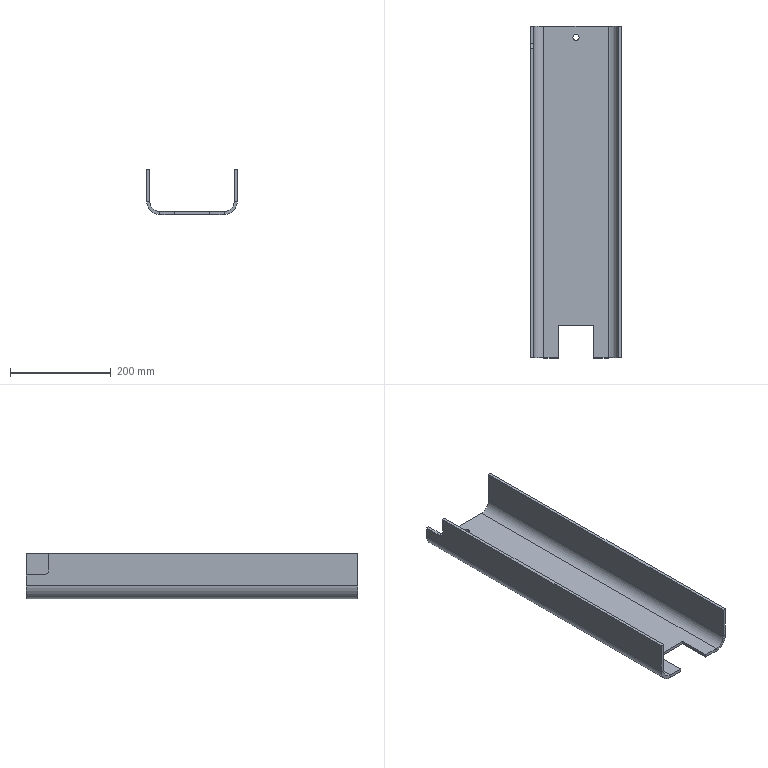Part | SolidWorks | features Cut 1, FlatPattern 1, SM3dBend 1, SMBaseFlange 1, SheetMetal 1 | 1 solid | 31 faces | box 180.012 x 660 x 89.996 mm | volume 1260450 mm3 | plane 24 | cylinder 7 | commonest cylinder face diameters 12 x2 40 x2 52 x2 20 x1
STEP:
#1=CARTESIAN_POINT('',(158.126,637.5,-6.));
#2=VERTEX_POINT('',#1);
#3=CARTESIAN_POINT('',(170.126,637.5,-6.));
#4=VERTEX_POINT('',#3);
#5=CARTESIAN_POINT('',(164.126,637.5,-6.));
#6=DIRECTION('',(0.,0.,1.));
#7=DIRECTION('',(1.,0.,0.));
#8=AXIS2_PLACEMENT_3D('',#5,#6,#7);
#9=CIRCLE('',#8,6.);
#10=EDGE_CURVE('',#2,#4,#9,.T.);
#11=ORIENTED_EDGE('',*,*,#10,.F.);
#12=CARTESIAN_POINT('',(158.126,637.5,0.));
#13=VERTEX_POINT('',#12);
#14=CARTESIAN_POINT('',(158.126,637.5,-6.));
#15=DIRECTION('',(0.,0.,1.));
#16=VECTOR('',#15,1000.);
#17=LINE('',#14,#16);
#18=EDGE_CURVE('',#2,#13,#17,.T.);
#19=ORIENTED_EDGE('',*,*,#18,.T.);
#20=CARTESIAN_POINT('',(170.126,637.5,0.));
#21=VERTEX_POINT('',#20);
#22=CARTESIAN_POINT('',(164.126,637.5,0.));
#23=DIRECTION('',(0.,0.,1.));
#24=DIRECTION('',(1.,0.,0.));
#25=AXIS2_PLACEMENT_3D('',#22,#23,#24);
#26=CIRCLE('',#25,6.);
#27=EDGE_CURVE('',#13,#21,#26,.T.);
#28=ORIENTED_EDGE('',*,*,#27,.T.);
#29=CARTESIAN_POINT('',(170.126,637.5,-6.));
#30=DIRECTION('',(0.,0.,1.));
#31=VECTOR('',#30,1000.);
#32=LINE('',#29,#31);
#33=EDGE_CURVE('',#4,#21,#32,.T.);
#34=ORIENTED_EDGE('',*,*,#33,.F.);
#35=EDGE_LOOP('',(#11,#19,#28,#34));
#36=FACE_OUTER_BOUND('',#35,.T.);
#37=CARTESIAN_POINT('',(164.126,637.5,-6.));
#38=DIRECTION('',(0.,0.,1.));
#39=DIRECTION('',(1.,0.,0.));
#40=AXIS2_PLACEMENT_3D('',#37,#38,#39);
#41=CYLINDRICAL_SURFACE('',#40,6.);
#42=ADVANCED_FACE('',(#36),#41,.F.);
#43=CARTESIAN_POINT('',(164.126,637.5,-6.));
#44=DIRECTION('',(0.,0.,1.));
#45=DIRECTION('',(1.,0.,0.));
#46=AXIS2_PLACEMENT_3D('',#43,#44,#45);
#47=CIRCLE('',#46,6.);
#48=EDGE_CURVE('',#4,#2,#47,.T.);
#49=ORIENTED_EDGE('',*,*,#48,.T.);
#50=ORIENTED_EDGE('',*,*,#10,.T.);
#51=EDGE_LOOP('',(#49,#50));
#52=FACE_BOUND('',#51,.T.);
#53=CARTESIAN_POINT('',(228.136,660.,-6.));
#54=VERTEX_POINT('',#53);
#55=CARTESIAN_POINT('',(100.124,660.,-6.));
#56=VERTEX_POINT('',#55);
#57=CARTESIAN_POINT('',(328.26,660.,-6.));
#58=DIRECTION('',(-1.,0.,0.));
#59=VECTOR('',#58,1000.);
#60=LINE('',#57,#59);
#61=EDGE_CURVE('',#54,#56,#60,.T.);
#62=ORIENTED_EDGE('',*,*,#61,.F.);
#63=CARTESIAN_POINT('',(228.136,0.,-6.));
#64=VERTEX_POINT('',#63);
#65=CARTESIAN_POINT('',(228.136,625.,-6.));
#66=DIRECTION('',(0.,-1.,0.));
#67=VECTOR('',#66,1000.);
#68=LINE('',#65,#67);
#69=EDGE_CURVE('',#54,#64,#68,.T.);
#70=ORIENTED_EDGE('',*,*,#69,.T.);
#71=CARTESIAN_POINT('',(199.13,0.,-6.));
#72=VERTEX_POINT('',#71);
#73=CARTESIAN_POINT('',(199.13,0.,-6.));
#74=DIRECTION('',(1.,0.,0.));
#75=VECTOR('',#74,1000.);
#76=LINE('',#73,#75);
#77=EDGE_CURVE('',#72,#64,#76,.T.);
#78=ORIENTED_EDGE('',*,*,#77,.F.);
#79=CARTESIAN_POINT('',(199.13,65.,-6.));
#80=VERTEX_POINT('',#79);
#81=CARTESIAN_POINT('',(199.13,0.,-6.));
#82=DIRECTION('',(0.,-1.,0.));
#83=VECTOR('',#82,1000.);
#84=LINE('',#81,#83);
#85=EDGE_CURVE('',#80,#72,#84,.T.);
#86=ORIENTED_EDGE('',*,*,#85,.F.);
#87=CARTESIAN_POINT('',(129.13,65.,-6.));
#88=VERTEX_POINT('',#87);
#89=CARTESIAN_POINT('',(199.13,65.,-6.));
#90=DIRECTION('',(1.,0.,0.));
#91=VECTOR('',#90,1000.);
#92=LINE('',#89,#91);
#93=EDGE_CURVE('',#88,#80,#92,.T.);
#94=ORIENTED_EDGE('',*,*,#93,.F.);
#95=CARTESIAN_POINT('',(129.13,0.,-6.));
#96=VERTEX_POINT('',#95);
#97=CARTESIAN_POINT('',(129.13,65.,-6.));
#98=DIRECTION('',(0.,1.,0.));
#99=VECTOR('',#98,1000.);
#100=LINE('',#97,#99);
#101=EDGE_CURVE('',#96,#88,#100,.T.);
#102=ORIENTED_EDGE('',*,*,#101,.F.);
#103=CARTESIAN_POINT('',(100.124,0.,-6.));
#104=VERTEX_POINT('',#103);
#105=CARTESIAN_POINT('',(0.,0.,-6.));
#106=DIRECTION('',(1.,0.,0.));
#107=VECTOR('',#106,1000.);
#108=LINE('',#105,#107);
#109=EDGE_CURVE('',#104,#96,#108,.T.);
#110=ORIENTED_EDGE('',*,*,#109,.F.);
#111=CARTESIAN_POINT('',(100.124,625.,-6.));
#112=DIRECTION('',(0.,-1.,0.));
#113=VECTOR('',#112,1000.);
#114=LINE('',#111,#113);
#115=EDGE_CURVE('',#56,#104,#114,.T.);
#116=ORIENTED_EDGE('',*,*,#115,.F.);
#117=EDGE_LOOP('',(#62,#70,#78,#86,#94,#102,#110,#116));
#118=FACE_OUTER_BOUND('',#117,.T.);
#119=CARTESIAN_POINT('',(33.,625.,-6.));
#120=DIRECTION('',(0.,0.,1.));
#121=DIRECTION('',(1.,0.,0.));
#122=AXIS2_PLACEMENT_3D('',#119,#120,#121);
#123=PLANE('',#122);
#124=ADVANCED_FACE('',(#52,#118),#123,.F.);
#125=CARTESIAN_POINT('',(228.136,660.,0.));
#126=VERTEX_POINT('',#125);
#127=CARTESIAN_POINT('',(228.136,660.,-6.));
#128=DIRECTION('',(0.,0.,1.));
#129=VECTOR('',#128,1000.);
#130=LINE('',#127,#129);
#131=EDGE_CURVE('',#54,#126,#130,.T.);
#132=ORIENTED_EDGE('',*,*,#131,.F.);
#133=ORIENTED_EDGE('',*,*,#61,.T.);
#134=CARTESIAN_POINT('',(100.124,660.,0.));
#135=VERTEX_POINT('',#134);
#136=CARTESIAN_POINT('',(100.124,660.,-6.));
#137=DIRECTION('',(0.,0.,1.));
#138=VECTOR('',#137,1000.);
#139=LINE('',#136,#138);
#140=EDGE_CURVE('',#56,#135,#139,.T.);
#141=ORIENTED_EDGE('',*,*,#140,.T.);
#142=CARTESIAN_POINT('',(328.26,660.,0.));
#143=DIRECTION('',(-1.,0.,0.));
#144=VECTOR('',#143,1000.);
#145=LINE('',#142,#144);
#146=EDGE_CURVE('',#126,#135,#145,.T.);
#147=ORIENTED_EDGE('',*,*,#146,.F.);
#148=EDGE_LOOP('',(#132,#133,#141,#147));
#149=FACE_OUTER_BOUND('',#148,.T.);
#150=CARTESIAN_POINT('',(328.26,660.,-6.));
#151=DIRECTION('',(0.,1.,0.));
#152=DIRECTION('',(0.,0.,1.));
#153=AXIS2_PLACEMENT_3D('',#150,#151,#152);
#154=PLANE('',#153);
#155=ADVANCED_FACE('',(#149),#154,.T.);
#156=CARTESIAN_POINT('',(100.124,0.,0.));
#157=VERTEX_POINT('',#156);
#158=CARTESIAN_POINT('',(129.13,0.,0.));
#159=VERTEX_POINT('',#158);
#160=CARTESIAN_POINT('',(0.,0.,0.));
#161=DIRECTION('',(1.,0.,0.));
#162=VECTOR('',#161,1000.);
#163=LINE('',#160,#162);
#164=EDGE_CURVE('',#157,#159,#163,.T.);
#165=ORIENTED_EDGE('',*,*,#164,.F.);
#166=CARTESIAN_POINT('',(100.124,0.,-6.));
#167=DIRECTION('',(0.,0.,-1.));
#168=VECTOR('',#167,1000.);
#169=LINE('',#166,#168);
#170=EDGE_CURVE('',#157,#104,#169,.T.);
#171=ORIENTED_EDGE('',*,*,#170,.T.);
#172=ORIENTED_EDGE('',*,*,#109,.T.);
#173=CARTESIAN_POINT('',(129.13,0.,-6.));
#174=DIRECTION('',(0.,0.,1.));
#175=VECTOR('',#174,1000.);
#176=LINE('',#173,#175);
#177=EDGE_CURVE('',#96,#159,#176,.T.);
#178=ORIENTED_EDGE('',*,*,#177,.T.);
#179=EDGE_LOOP('',(#165,#171,#172,#178));
#180=FACE_OUTER_BOUND('',#179,.T.);
#181=CARTESIAN_POINT('',(0.,0.,-6.));
#182=DIRECTION('',(0.,-1.,0.));
#183=DIRECTION('',(0.,0.,-1.));
#184=AXIS2_PLACEMENT_3D('',#181,#182,#183);
#185=PLANE('',#184);
#186=ADVANCED_FACE('',(#180),#185,.T.);
#187=CARTESIAN_POINT('',(164.126,637.5,0.));
#188=DIRECTION('',(0.,0.,1.));
#189=DIRECTION('',(1.,0.,0.));
#190=AXIS2_PLACEMENT_3D('',#187,#188,#189);
#191=CIRCLE('',#190,6.);
#192=EDGE_CURVE('',#21,#13,#191,.T.);
#193=ORIENTED_EDGE('',*,*,#192,.F.);
#194=ORIENTED_EDGE('',*,*,#27,.F.);
#195=EDGE_LOOP('',(#193,#194));
#196=FACE_BOUND('',#195,.T.);
#197=CARTESIAN_POINT('',(228.136,0.,0.));
#198=VERTEX_POINT('',#197);
#199=CARTESIAN_POINT('',(228.136,625.,0.));
#200=DIRECTION('',(0.,-1.,0.));
#201=VECTOR('',#200,1000.);
#202=LINE('',#199,#201);
#203=EDGE_CURVE('',#126,#198,#202,.T.);
#204=ORIENTED_EDGE('',*,*,#203,.F.);
#205=ORIENTED_EDGE('',*,*,#146,.T.);
#206=CARTESIAN_POINT('',(100.124,625.,0.));
#207=DIRECTION('',(0.,-1.,0.));
#208=VECTOR('',#207,1000.);
#209=LINE('',#206,#208);
#210=EDGE_CURVE('',#135,#157,#209,.T.);
#211=ORIENTED_EDGE('',*,*,#210,.T.);
#212=ORIENTED_EDGE('',*,*,#164,.T.);
#213=CARTESIAN_POINT('',(129.13,65.,0.));
#214=VERTEX_POINT('',#213);
#215=CARTESIAN_POINT('',(129.13,65.,0.));
#216=DIRECTION('',(0.,1.,0.));
#217=VECTOR('',#216,1000.);
#218=LINE('',#215,#217);
#219=EDGE_CURVE('',#159,#214,#218,.T.);
#220=ORIENTED_EDGE('',*,*,#219,.T.);
#221=CARTESIAN_POINT('',(199.13,65.,0.));
#222=VERTEX_POINT('',#221);
#223=CARTESIAN_POINT('',(199.13,65.,0.));
#224=DIRECTION('',(1.,0.,0.));
#225=VECTOR('',#224,1000.);
#226=LINE('',#223,#225);
#227=EDGE_CURVE('',#214,#222,#226,.T.);
#228=ORIENTED_EDGE('',*,*,#227,.T.);
#229=CARTESIAN_POINT('',(199.13,0.,0.));
#230=VERTEX_POINT('',#229);
#231=CARTESIAN_POINT('',(199.13,0.,0.));
#232=DIRECTION('',(0.,-1.,0.));
#233=VECTOR('',#232,1000.);
#234=LINE('',#231,#233);
#235=EDGE_CURVE('',#222,#230,#234,.T.);
#236=ORIENTED_EDGE('',*,*,#235,.T.);
#237=CARTESIAN_POINT('',(199.13,0.,0.));
#238=DIRECTION('',(1.,0.,0.));
#239=VECTOR('',#238,1000.);
#240=LINE('',#237,#239);
#241=EDGE_CURVE('',#230,#198,#240,.T.);
#242=ORIENTED_EDGE('',*,*,#241,.T.);
#243=EDGE_LOOP('',(#204,#205,#211,#212,#220,#228,#236,#242));
#244=FACE_OUTER_BOUND('',#243,.T.);
#245=CARTESIAN_POINT('',(33.,625.,0.));
#246=DIRECTION('',(0.,0.,1.));
#247=DIRECTION('',(1.,0.,0.));
#248=AXIS2_PLACEMENT_3D('',#245,#246,#247);
#249=PLANE('',#248);
#250=ADVANCED_FACE('',(#196,#244),#249,.T.);
#251=CARTESIAN_POINT('',(228.136,0.,-6.));
#252=DIRECTION('',(0.,0.,-1.));
#253=VECTOR('',#252,1000.);
#254=LINE('',#251,#253);
#255=EDGE_CURVE('',#198,#64,#254,.T.);
#256=ORIENTED_EDGE('',*,*,#255,.F.);
#257=ORIENTED_EDGE('',*,*,#241,.F.);
#258=CARTESIAN_POINT('',(199.13,0.,-6.));
#259=DIRECTION('',(0.,0.,1.));
#260=VECTOR('',#259,1000.);
#261=LINE('',#258,#260);
#262=EDGE_CURVE('',#72,#230,#261,.T.);
#263=ORIENTED_EDGE('',*,*,#262,.F.);
#264=ORIENTED_EDGE('',*,*,#77,.T.);
#265=EDGE_LOOP('',(#256,#257,#263,#264));
#266=FACE_OUTER_BOUND('',#265,.T.);
#267=CARTESIAN_POINT('',(199.13,0.,-6.));
#268=DIRECTION('',(0.,-1.,0.));
#269=DIRECTION('',(0.,0.,-1.));
#270=AXIS2_PLACEMENT_3D('',#267,#268,#269);
#271=PLANE('',#270);
#272=ADVANCED_FACE('',(#266),#271,.T.);
#273=ORIENTED_EDGE('',*,*,#235,.F.);
#274=CARTESIAN_POINT('',(199.13,65.,-6.));
#275=DIRECTION('',(0.,0.,1.));
#276=VECTOR('',#275,1000.);
#277=LINE('',#274,#276);
#278=EDGE_CURVE('',#80,#222,#277,.T.);
#279=ORIENTED_EDGE('',*,*,#278,.F.);
#280=ORIENTED_EDGE('',*,*,#85,.T.);
#281=ORIENTED_EDGE('',*,*,#262,.T.);
#282=EDGE_LOOP('',(#273,#279,#280,#281));
#283=FACE_OUTER_BOUND('',#282,.T.);
#284=CARTESIAN_POINT('',(199.13,0.,-6.));
#285=DIRECTION('',(-1.,0.,0.));
#286=DIRECTION('',(0.,0.,1.));
#287=AXIS2_PLACEMENT_3D('',#284,#285,#286);
#288=PLANE('',#287);
#289=ADVANCED_FACE('',(#283),#288,.T.);
#290=ORIENTED_EDGE('',*,*,#227,.F.);
#291=CARTESIAN_POINT('',(129.13,65.,-6.));
#292=DIRECTION('',(0.,0.,1.));
#293=VECTOR('',#292,1000.);
#294=LINE('',#291,#293);
#295=EDGE_CURVE('',#88,#214,#294,.T.);
#296=ORIENTED_EDGE('',*,*,#295,.F.);
#297=ORIENTED_EDGE('',*,*,#93,.T.);
#298=ORIENTED_EDGE('',*,*,#278,.T.);
#299=EDGE_LOOP('',(#290,#296,#297,#298));
#300=FACE_OUTER_BOUND('',#299,.T.);
#301=CARTESIAN_POINT('',(199.13,65.,-6.));
#302=DIRECTION('',(0.,-1.,0.));
#303=DIRECTION('',(1.,0.,0.));
#304=AXIS2_PLACEMENT_3D('',#301,#302,#303);
#305=PLANE('',#304);
#306=ADVANCED_FACE('',(#300),#305,.T.);
#307=ORIENTED_EDGE('',*,*,#219,.F.);
#308=ORIENTED_EDGE('',*,*,#177,.F.);
#309=ORIENTED_EDGE('',*,*,#101,.T.);
#310=ORIENTED_EDGE('',*,*,#295,.T.);
#311=EDGE_LOOP('',(#307,#308,#309,#310));
#312=FACE_OUTER_BOUND('',#311,.T.);
#313=CARTESIAN_POINT('',(129.13,65.,-6.));
#314=DIRECTION('',(1.,0.,0.));
#315=DIRECTION('',(0.,0.,-1.));
#316=AXIS2_PLACEMENT_3D('',#313,#314,#315);
#317=PLANE('',#316);
#318=ADVANCED_FACE('',(#312),#317,.T.);
#319=CARTESIAN_POINT('',(74.124,660.,20.));
#320=VERTEX_POINT('',#319);
#321=CARTESIAN_POINT('',(80.124,660.,20.));
#322=VERTEX_POINT('',#321);
#323=CARTESIAN_POINT('',(74.124,660.,20.));
#324=DIRECTION('',(1.,0.,0.));
#325=VECTOR('',#324,1000.);
#326=LINE('',#323,#325);
#327=EDGE_CURVE('',#320,#322,#326,.T.);
#328=ORIENTED_EDGE('',*,*,#327,.T.);
#329=CARTESIAN_POINT('',(100.124,660.,20.));
#330=DIRECTION('',(0.,-1.,0.));
#331=DIRECTION('',(0.,0.,1.));
#332=AXIS2_PLACEMENT_3D('',#329,#330,#331);
#333=CIRCLE('',#332,20.);
#334=EDGE_CURVE('',#322,#135,#333,.T.);
#335=ORIENTED_EDGE('',*,*,#334,.T.);
#336=ORIENTED_EDGE('',*,*,#140,.F.);
#337=CARTESIAN_POINT('',(100.124,660.,20.));
#338=DIRECTION('',(0.,-1.,0.));
#339=DIRECTION('',(0.,0.,1.));
#340=AXIS2_PLACEMENT_3D('',#337,#338,#339);
#341=CIRCLE('',#340,26.);
#342=EDGE_CURVE('',#320,#56,#341,.T.);
#343=ORIENTED_EDGE('',*,*,#342,.F.);
#344=EDGE_LOOP('',(#328,#335,#336,#343));
#345=FACE_OUTER_BOUND('',#344,.T.);
#346=CARTESIAN_POINT('',(100.124,660.,20.));
#347=DIRECTION('',(0.,1.,0.));
#348=DIRECTION('',(0.,0.,1.));
#349=AXIS2_PLACEMENT_3D('',#346,#347,#348);
#350=PLANE('',#349);
#351=ADVANCED_FACE('',(#345),#350,.T.);
#352=ORIENTED_EDGE('',*,*,#170,.F.);
#353=CARTESIAN_POINT('',(80.124,0.,20.));
#354=VERTEX_POINT('',#353);
#355=CARTESIAN_POINT('',(100.124,0.,20.));
#356=DIRECTION('',(0.,1.,0.));
#357=DIRECTION('',(0.,0.,1.));
#358=AXIS2_PLACEMENT_3D('',#355,#356,#357);
#359=CIRCLE('',#358,20.);
#360=EDGE_CURVE('',#157,#354,#359,.T.);
#361=ORIENTED_EDGE('',*,*,#360,.T.);
#362=CARTESIAN_POINT('',(74.124,0.,20.));
#363=VERTEX_POINT('',#362);
#364=CARTESIAN_POINT('',(74.124,0.,20.));
#365=DIRECTION('',(-1.,0.,0.));
#366=VECTOR('',#365,1000.);
#367=LINE('',#364,#366);
#368=EDGE_CURVE('',#354,#363,#367,.T.);
#369=ORIENTED_EDGE('',*,*,#368,.T.);
#370=CARTESIAN_POINT('',(100.124,0.,20.));
#371=DIRECTION('',(0.,1.,0.));
#372=DIRECTION('',(0.,0.,-1.));
#373=AXIS2_PLACEMENT_3D('',#370,#371,#372);
#374=CIRCLE('',#373,26.);
#375=EDGE_CURVE('',#104,#363,#374,.T.);
#376=ORIENTED_EDGE('',*,*,#375,.F.);
#377=EDGE_LOOP('',(#352,#361,#369,#376));
#378=FACE_OUTER_BOUND('',#377,.T.);
#379=CARTESIAN_POINT('',(100.124,0.,20.));
#380=DIRECTION('',(0.,-1.,0.));
#381=DIRECTION('',(0.,0.,-1.));
#382=AXIS2_PLACEMENT_3D('',#379,#380,#381);
#383=PLANE('',#382);
#384=ADVANCED_FACE('',(#378),#383,.T.);
#385=ORIENTED_EDGE('',*,*,#375,.T.);
#386=CARTESIAN_POINT('',(74.124,625.,20.));
#387=DIRECTION('',(0.,-1.,0.));
#388=VECTOR('',#387,1000.);
#389=LINE('',#386,#388);
#390=EDGE_CURVE('',#320,#363,#389,.T.);
#391=ORIENTED_EDGE('',*,*,#390,.F.);
#392=ORIENTED_EDGE('',*,*,#342,.T.);
#393=ORIENTED_EDGE('',*,*,#115,.T.);
#394=EDGE_LOOP('',(#385,#391,#392,#393));
#395=FACE_OUTER_BOUND('',#394,.T.);
#396=CARTESIAN_POINT('',(100.124,-331.015,20.));
#397=DIRECTION('',(0.,1.,0.));
#398=DIRECTION('',(0.,0.,1.));
#399=AXIS2_PLACEMENT_3D('',#396,#397,#398);
#400=CYLINDRICAL_SURFACE('',#399,26.);
#401=ADVANCED_FACE('',(#395),#400,.T.);
#402=ORIENTED_EDGE('',*,*,#360,.F.);
#403=ORIENTED_EDGE('',*,*,#210,.F.);
#404=ORIENTED_EDGE('',*,*,#334,.F.);
#405=CARTESIAN_POINT('',(80.124,625.,20.));
#406=DIRECTION('',(0.,-1.,0.));
#407=VECTOR('',#406,1000.);
#408=LINE('',#405,#407);
#409=EDGE_CURVE('',#322,#354,#408,.T.);
#410=ORIENTED_EDGE('',*,*,#409,.T.);
#411=EDGE_LOOP('',(#402,#403,#404,#410));
#412=FACE_OUTER_BOUND('',#411,.T.);
#413=CARTESIAN_POINT('',(100.124,-331.015,20.));
#414=DIRECTION('',(0.,1.,0.));
#415=DIRECTION('',(0.,0.,1.));
#416=AXIS2_PLACEMENT_3D('',#413,#414,#415);
#417=CYLINDRICAL_SURFACE('',#416,20.);
#418=ADVANCED_FACE('',(#412),#417,.F.);
#419=CARTESIAN_POINT('',(80.124,660.,40.996));
#420=VERTEX_POINT('',#419);
#421=CARTESIAN_POINT('',(80.124,625.,40.996));
#422=VERTEX_POINT('',#421);
#423=CARTESIAN_POINT('',(80.124,625.,40.996));
#424=DIRECTION('',(0.,-1.,0.));
#425=VECTOR('',#424,1000.);
#426=LINE('',#423,#425);
#427=EDGE_CURVE('',#420,#422,#426,.T.);
#428=ORIENTED_EDGE('',*,*,#427,.F.);
#429=CARTESIAN_POINT('',(74.124,660.,40.996));
#430=VERTEX_POINT('',#429);
#431=CARTESIAN_POINT('',(74.124,660.,40.996));
#432=DIRECTION('',(1.,0.,0.));
#433=VECTOR('',#432,1000.);
#434=LINE('',#431,#433);
#435=EDGE_CURVE('',#430,#420,#434,.T.);
#436=ORIENTED_EDGE('',*,*,#435,.F.);
#437=CARTESIAN_POINT('',(74.124,625.,40.996));
#438=VERTEX_POINT('',#437);
#439=CARTESIAN_POINT('',(74.124,625.,40.996));
#440=DIRECTION('',(0.,-1.,0.));
#441=VECTOR('',#440,1000.);
#442=LINE('',#439,#441);
#443=EDGE_CURVE('',#430,#438,#442,.T.);
#444=ORIENTED_EDGE('',*,*,#443,.T.);
#445=CARTESIAN_POINT('',(74.124,625.,40.996));
#446=DIRECTION('',(1.,0.,0.));
#447=VECTOR('',#446,1000.);
#448=LINE('',#445,#447);
#449=EDGE_CURVE('',#438,#422,#448,.T.);
#450=ORIENTED_EDGE('',*,*,#449,.T.);
#451=EDGE_LOOP('',(#428,#436,#444,#450));
#452=FACE_OUTER_BOUND('',#451,.T.);
#453=CARTESIAN_POINT('',(74.124,625.,40.996));
#454=DIRECTION('',(0.,0.,1.));
#455=DIRECTION('',(0.,-1.,0.));
#456=AXIS2_PLACEMENT_3D('',#453,#454,#455);
#457=PLANE('',#456);
#458=ADVANCED_FACE('',(#452),#457,.T.);
#459=CARTESIAN_POINT('',(80.124,615.,50.996));
#460=VERTEX_POINT('',#459);
#461=CARTESIAN_POINT('',(80.124,625.,50.996));
#462=DIRECTION('',(-1.,0.,0.));
#463=DIRECTION('',(0.,0.,-1.));
#464=AXIS2_PLACEMENT_3D('',#461,#462,#463);
#465=CIRCLE('',#464,10.);
#466=EDGE_CURVE('',#422,#460,#465,.T.);
#467=ORIENTED_EDGE('',*,*,#466,.F.);
#468=ORIENTED_EDGE('',*,*,#449,.F.);
#469=CARTESIAN_POINT('',(74.124,615.,50.996));
#470=VERTEX_POINT('',#469);
#471=CARTESIAN_POINT('',(74.124,625.,50.996));
#472=DIRECTION('',(-1.,0.,0.));
#473=DIRECTION('',(0.,0.,-1.));
#474=AXIS2_PLACEMENT_3D('',#471,#472,#473);
#475=CIRCLE('',#474,10.);
#476=EDGE_CURVE('',#438,#470,#475,.T.);
#477=ORIENTED_EDGE('',*,*,#476,.T.);
#478=CARTESIAN_POINT('',(74.124,615.,50.996));
#479=DIRECTION('',(1.,0.,0.));
#480=VECTOR('',#479,1000.);
#481=LINE('',#478,#480);
#482=EDGE_CURVE('',#470,#460,#481,.T.);
#483=ORIENTED_EDGE('',*,*,#482,.T.);
#484=EDGE_LOOP('',(#467,#468,#477,#483));
#485=FACE_OUTER_BOUND('',#484,.T.);
#486=CARTESIAN_POINT('',(74.124,625.,50.996));
#487=DIRECTION('',(1.,0.,0.));
#488=DIRECTION('',(0.,0.,-1.));
#489=AXIS2_PLACEMENT_3D('',#486,#487,#488);
#490=CYLINDRICAL_SURFACE('',#489,10.);
#491=ADVANCED_FACE('',(#485),#490,.F.);
#492=CARTESIAN_POINT('',(80.124,615.,83.996));
#493=VERTEX_POINT('',#492);
#494=CARTESIAN_POINT('',(80.124,615.,83.996));
#495=DIRECTION('',(0.,0.,1.));
#496=VECTOR('',#495,1000.);
#497=LINE('',#494,#496);
#498=EDGE_CURVE('',#460,#493,#497,.T.);
#499=ORIENTED_EDGE('',*,*,#498,.F.);
#500=ORIENTED_EDGE('',*,*,#482,.F.);
#501=CARTESIAN_POINT('',(74.124,615.,83.996));
#502=VERTEX_POINT('',#501);
#503=CARTESIAN_POINT('',(74.124,615.,83.996));
#504=DIRECTION('',(0.,0.,1.));
#505=VECTOR('',#504,1000.);
#506=LINE('',#503,#505);
#507=EDGE_CURVE('',#470,#502,#506,.T.);
#508=ORIENTED_EDGE('',*,*,#507,.T.);
#509=CARTESIAN_POINT('',(74.124,615.,83.996));
#510=DIRECTION('',(1.,0.,0.));
#511=VECTOR('',#510,1000.);
#512=LINE('',#509,#511);
#513=EDGE_CURVE('',#502,#493,#512,.T.);
#514=ORIENTED_EDGE('',*,*,#513,.T.);
#515=EDGE_LOOP('',(#499,#500,#508,#514));
#516=FACE_OUTER_BOUND('',#515,.T.);
#517=CARTESIAN_POINT('',(74.124,615.,83.996));
#518=DIRECTION('',(0.,1.,0.));
#519=DIRECTION('',(1.,0.,0.));
#520=AXIS2_PLACEMENT_3D('',#517,#518,#519);
#521=PLANE('',#520);
#522=ADVANCED_FACE('',(#516),#521,.T.);
#523=CARTESIAN_POINT('',(80.124,0.,83.996));
#524=VERTEX_POINT('',#523);
#525=CARTESIAN_POINT('',(80.124,615.,83.996));
#526=DIRECTION('',(0.,-1.,0.));
#527=VECTOR('',#526,1000.);
#528=LINE('',#525,#527);
#529=EDGE_CURVE('',#493,#524,#528,.T.);
#530=ORIENTED_EDGE('',*,*,#529,.F.);
#531=ORIENTED_EDGE('',*,*,#513,.F.);
#532=CARTESIAN_POINT('',(74.124,0.,83.996));
#533=VERTEX_POINT('',#532);
#534=CARTESIAN_POINT('',(74.124,615.,83.996));
#535=DIRECTION('',(0.,-1.,0.));
#536=VECTOR('',#535,1000.);
#537=LINE('',#534,#536);
#538=EDGE_CURVE('',#502,#533,#537,.T.);
#539=ORIENTED_EDGE('',*,*,#538,.T.);
#540=CARTESIAN_POINT('',(74.124,0.,83.996));
#541=DIRECTION('',(1.,0.,0.));
#542=VECTOR('',#541,1000.);
#543=LINE('',#540,#542);
#544=EDGE_CURVE('',#533,#524,#543,.T.);
#545=ORIENTED_EDGE('',*,*,#544,.T.);
#546=EDGE_LOOP('',(#530,#531,#539,#545));
#547=FACE_OUTER_BOUND('',#546,.T.);
#548=CARTESIAN_POINT('',(74.124,615.,83.996));
#549=DIRECTION('',(0.,0.,1.));
#550=DIRECTION('',(0.,-1.,0.));
#551=AXIS2_PLACEMENT_3D('',#548,#549,#550);
#552=PLANE('',#551);
#553=ADVANCED_FACE('',(#547),#552,.T.);
#554=CARTESIAN_POINT('',(74.124,660.,-244.264));
#555=DIRECTION('',(0.,0.,1.));
#556=VECTOR('',#555,1000.);
#557=LINE('',#554,#556);
#558=EDGE_CURVE('',#320,#430,#557,.T.);
#559=ORIENTED_EDGE('',*,*,#558,.F.);
#560=ORIENTED_EDGE('',*,*,#390,.T.);
#561=CARTESIAN_POINT('',(74.124,0.,83.996));
#562=DIRECTION('',(0.,0.,-1.));
#563=VECTOR('',#562,1000.);
#564=LINE('',#561,#563);
#565=EDGE_CURVE('',#533,#363,#564,.T.);
#566=ORIENTED_EDGE('',*,*,#565,.F.);
#567=ORIENTED_EDGE('',*,*,#538,.F.);
#568=ORIENTED_EDGE('',*,*,#507,.F.);
#569=ORIENTED_EDGE('',*,*,#476,.F.);
#570=ORIENTED_EDGE('',*,*,#443,.F.);
#571=EDGE_LOOP('',(#559,#560,#566,#567,#568,#569,#570));
#572=FACE_OUTER_BOUND('',#571,.T.);
#573=CARTESIAN_POINT('',(74.124,625.,50.996));
#574=DIRECTION('',(1.,0.,0.));
#575=DIRECTION('',(0.,0.,-1.));
#576=AXIS2_PLACEMENT_3D('',#573,#574,#575);
#577=PLANE('',#576);
#578=ADVANCED_FACE('',(#572),#577,.F.);
#579=ORIENTED_EDGE('',*,*,#368,.F.);
#580=CARTESIAN_POINT('',(80.124,0.,83.996));
#581=DIRECTION('',(0.,0.,-1.));
#582=VECTOR('',#581,1000.);
#583=LINE('',#580,#582);
#584=EDGE_CURVE('',#524,#354,#583,.T.);
#585=ORIENTED_EDGE('',*,*,#584,.F.);
#586=ORIENTED_EDGE('',*,*,#544,.F.);
#587=ORIENTED_EDGE('',*,*,#565,.T.);
#588=EDGE_LOOP('',(#579,#585,#586,#587));
#589=FACE_OUTER_BOUND('',#588,.T.);
#590=CARTESIAN_POINT('',(74.124,0.,83.996));
#591=DIRECTION('',(0.,-1.,0.));
#592=DIRECTION('',(-1.,0.,0.));
#593=AXIS2_PLACEMENT_3D('',#590,#591,#592);
#594=PLANE('',#593);
#595=ADVANCED_FACE('',(#589),#594,.T.);
#596=ORIENTED_EDGE('',*,*,#409,.F.);
#597=CARTESIAN_POINT('',(80.124,660.,-244.264));
#598=DIRECTION('',(0.,0.,1.));
#599=VECTOR('',#598,1000.);
#600=LINE('',#597,#599);
#601=EDGE_CURVE('',#322,#420,#600,.T.);
#602=ORIENTED_EDGE('',*,*,#601,.T.);
#603=ORIENTED_EDGE('',*,*,#427,.T.);
#604=ORIENTED_EDGE('',*,*,#466,.T.);
#605=ORIENTED_EDGE('',*,*,#498,.T.);
#606=ORIENTED_EDGE('',*,*,#529,.T.);
#607=ORIENTED_EDGE('',*,*,#584,.T.);
#608=EDGE_LOOP('',(#596,#602,#603,#604,#605,#606,#607));
#609=FACE_OUTER_BOUND('',#608,.T.);
#610=CARTESIAN_POINT('',(80.124,625.,50.996));
#611=DIRECTION('',(1.,0.,0.));
#612=DIRECTION('',(0.,0.,-1.));
#613=AXIS2_PLACEMENT_3D('',#610,#611,#612);
#614=PLANE('',#613);
#615=ADVANCED_FACE('',(#609),#614,.T.);
#616=ORIENTED_EDGE('',*,*,#327,.F.);
#617=ORIENTED_EDGE('',*,*,#558,.T.);
#618=ORIENTED_EDGE('',*,*,#435,.T.);
#619=ORIENTED_EDGE('',*,*,#601,.F.);
#620=EDGE_LOOP('',(#616,#617,#618,#619));
#621=FACE_OUTER_BOUND('',#620,.T.);
#622=CARTESIAN_POINT('',(74.124,660.,-244.264));
#623=DIRECTION('',(0.,1.,0.));
#624=DIRECTION('',(1.,0.,0.));
#625=AXIS2_PLACEMENT_3D('',#622,#623,#624);
#626=PLANE('',#625);
#627=ADVANCED_FACE('',(#621),#626,.T.);
#628=ORIENTED_EDGE('',*,*,#131,.T.);
#629=CARTESIAN_POINT('',(248.136,660.,20.));
#630=VERTEX_POINT('',#629);
#631=CARTESIAN_POINT('',(228.136,660.,20.));
#632=DIRECTION('',(0.,-1.,0.));
#633=DIRECTION('',(0.,0.,-1.));
#634=AXIS2_PLACEMENT_3D('',#631,#632,#633);
#635=CIRCLE('',#634,20.);
#636=EDGE_CURVE('',#126,#630,#635,.T.);
#637=ORIENTED_EDGE('',*,*,#636,.T.);
#638=CARTESIAN_POINT('',(254.136,660.,20.));
#639=VERTEX_POINT('',#638);
#640=CARTESIAN_POINT('',(254.136,660.,20.));
#641=DIRECTION('',(-1.,0.,0.));
#642=VECTOR('',#641,1000.);
#643=LINE('',#640,#642);
#644=EDGE_CURVE('',#639,#630,#643,.T.);
#645=ORIENTED_EDGE('',*,*,#644,.F.);
#646=CARTESIAN_POINT('',(228.136,660.,20.));
#647=DIRECTION('',(0.,-1.,0.));
#648=DIRECTION('',(0.,0.,1.));
#649=AXIS2_PLACEMENT_3D('',#646,#647,#648);
#650=CIRCLE('',#649,26.);
#651=EDGE_CURVE('',#54,#639,#650,.T.);
#652=ORIENTED_EDGE('',*,*,#651,.F.);
#653=EDGE_LOOP('',(#628,#637,#645,#652));
#654=FACE_OUTER_BOUND('',#653,.T.);
#655=CARTESIAN_POINT('',(228.136,660.,20.));
#656=DIRECTION('',(0.,1.,0.));
#657=DIRECTION('',(0.,0.,1.));
#658=AXIS2_PLACEMENT_3D('',#655,#656,#657);
#659=PLANE('',#658);
#660=ADVANCED_FACE('',(#654),#659,.T.);
#661=CARTESIAN_POINT('',(248.136,0.,20.));
#662=VERTEX_POINT('',#661);
#663=CARTESIAN_POINT('',(254.136,0.,20.));
#664=VERTEX_POINT('',#663);
#665=CARTESIAN_POINT('',(254.136,0.,20.));
#666=DIRECTION('',(1.,0.,0.));
#667=VECTOR('',#666,1000.);
#668=LINE('',#665,#667);
#669=EDGE_CURVE('',#662,#664,#668,.T.);
#670=ORIENTED_EDGE('',*,*,#669,.F.);
#671=CARTESIAN_POINT('',(228.136,0.,20.));
#672=DIRECTION('',(0.,1.,0.));
#673=DIRECTION('',(0.,0.,-1.));
#674=AXIS2_PLACEMENT_3D('',#671,#672,#673);
#675=CIRCLE('',#674,20.);
#676=EDGE_CURVE('',#662,#198,#675,.T.);
#677=ORIENTED_EDGE('',*,*,#676,.T.);
#678=ORIENTED_EDGE('',*,*,#255,.T.);
#679=CARTESIAN_POINT('',(228.136,0.,20.));
#680=DIRECTION('',(0.,1.,0.));
#681=DIRECTION('',(0.,0.,-1.));
#682=AXIS2_PLACEMENT_3D('',#679,#680,#681);
#683=CIRCLE('',#682,26.);
#684=EDGE_CURVE('',#664,#64,#683,.T.);
#685=ORIENTED_EDGE('',*,*,#684,.F.);
#686=EDGE_LOOP('',(#670,#677,#678,#685));
#687=FACE_OUTER_BOUND('',#686,.T.);
#688=CARTESIAN_POINT('',(228.136,0.,20.));
#689=DIRECTION('',(0.,-1.,0.));
#690=DIRECTION('',(0.,0.,-1.));
#691=AXIS2_PLACEMENT_3D('',#688,#689,#690);
#692=PLANE('',#691);
#693=ADVANCED_FACE('',(#687),#692,.T.);
#694=ORIENTED_EDGE('',*,*,#684,.T.);
#695=ORIENTED_EDGE('',*,*,#69,.F.);
#696=ORIENTED_EDGE('',*,*,#651,.T.);
#697=CARTESIAN_POINT('',(254.136,625.,20.));
#698=DIRECTION('',(0.,-1.,0.));
#699=VECTOR('',#698,1000.);
#700=LINE('',#697,#699);
#701=EDGE_CURVE('',#639,#664,#700,.T.);
#702=ORIENTED_EDGE('',*,*,#701,.T.);
#703=EDGE_LOOP('',(#694,#695,#696,#702));
#704=FACE_OUTER_BOUND('',#703,.T.);
#705=CARTESIAN_POINT('',(228.136,991.015,20.));
#706=DIRECTION('',(0.,-1.,0.));
#707=DIRECTION('',(0.,0.,-1.));
#708=AXIS2_PLACEMENT_3D('',#705,#706,#707);
#709=CYLINDRICAL_SURFACE('',#708,26.);
#710=ADVANCED_FACE('',(#704),#709,.T.);
#711=ORIENTED_EDGE('',*,*,#676,.F.);
#712=CARTESIAN_POINT('',(248.136,625.,20.));
#713=DIRECTION('',(0.,-1.,0.));
#714=VECTOR('',#713,1000.);
#715=LINE('',#712,#714);
#716=EDGE_CURVE('',#630,#662,#715,.T.);
#717=ORIENTED_EDGE('',*,*,#716,.F.);
#718=ORIENTED_EDGE('',*,*,#636,.F.);
#719=ORIENTED_EDGE('',*,*,#203,.T.);
#720=EDGE_LOOP('',(#711,#717,#718,#719));
#721=FACE_OUTER_BOUND('',#720,.T.);
#722=CARTESIAN_POINT('',(228.136,991.015,20.));
#723=DIRECTION('',(0.,-1.,0.));
#724=DIRECTION('',(0.,0.,-1.));
#725=AXIS2_PLACEMENT_3D('',#722,#723,#724);
#726=CYLINDRICAL_SURFACE('',#725,20.);
#727=ADVANCED_FACE('',(#721),#726,.F.);
#728=CARTESIAN_POINT('',(248.136,0.,83.996));
#729=VERTEX_POINT('',#728);
#730=CARTESIAN_POINT('',(248.136,660.,83.996));
#731=VERTEX_POINT('',#730);
#732=CARTESIAN_POINT('',(248.136,0.,83.996));
#733=DIRECTION('',(0.,1.,0.));
#734=VECTOR('',#733,1000.);
#735=LINE('',#732,#734);
#736=EDGE_CURVE('',#729,#731,#735,.T.);
#737=ORIENTED_EDGE('',*,*,#736,.F.);
#738=CARTESIAN_POINT('',(254.136,0.,83.996));
#739=VERTEX_POINT('',#738);
#740=CARTESIAN_POINT('',(254.136,0.,83.996));
#741=DIRECTION('',(-1.,0.,0.));
#742=VECTOR('',#741,1000.);
#743=LINE('',#740,#742);
#744=EDGE_CURVE('',#739,#729,#743,.T.);
#745=ORIENTED_EDGE('',*,*,#744,.F.);
#746=CARTESIAN_POINT('',(254.136,660.,83.996));
#747=VERTEX_POINT('',#746);
#748=CARTESIAN_POINT('',(254.136,0.,83.996));
#749=DIRECTION('',(0.,1.,0.));
#750=VECTOR('',#749,1000.);
#751=LINE('',#748,#750);
#752=EDGE_CURVE('',#739,#747,#751,.T.);
#753=ORIENTED_EDGE('',*,*,#752,.T.);
#754=CARTESIAN_POINT('',(254.136,660.,83.996));
#755=DIRECTION('',(-1.,0.,0.));
#756=VECTOR('',#755,1000.);
#757=LINE('',#754,#756);
#758=EDGE_CURVE('',#747,#731,#757,.T.);
#759=ORIENTED_EDGE('',*,*,#758,.T.);
#760=EDGE_LOOP('',(#737,#745,#753,#759));
#761=FACE_OUTER_BOUND('',#760,.T.);
#762=CARTESIAN_POINT('',(254.136,0.,83.996));
#763=DIRECTION('',(0.,0.,1.));
#764=DIRECTION('',(1.,0.,0.));
#765=AXIS2_PLACEMENT_3D('',#762,#763,#764);
#766=PLANE('',#765);
#767=ADVANCED_FACE('',(#761),#766,.T.);
#768=ORIENTED_EDGE('',*,*,#701,.F.);
#769=CARTESIAN_POINT('',(254.136,660.,83.996));
#770=DIRECTION('',(0.,0.,-1.));
#771=VECTOR('',#770,1000.);
#772=LINE('',#769,#771);
#773=EDGE_CURVE('',#747,#639,#772,.T.);
#774=ORIENTED_EDGE('',*,*,#773,.F.);
#775=ORIENTED_EDGE('',*,*,#752,.F.);
#776=CARTESIAN_POINT('',(254.136,0.,-45.134));
#777=DIRECTION('',(0.,0.,1.));
#778=VECTOR('',#777,1000.);
#779=LINE('',#776,#778);
#780=EDGE_CURVE('',#664,#739,#779,.T.);
#781=ORIENTED_EDGE('',*,*,#780,.F.);
#782=EDGE_LOOP('',(#768,#774,#775,#781));
#783=FACE_OUTER_BOUND('',#782,.T.);
#784=CARTESIAN_POINT('',(254.136,625.,-211.264));
#785=DIRECTION('',(-1.,0.,0.));
#786=DIRECTION('',(0.,0.,1.));
#787=AXIS2_PLACEMENT_3D('',#784,#785,#786);
#788=PLANE('',#787);
#789=ADVANCED_FACE('',(#783),#788,.F.);
#790=ORIENTED_EDGE('',*,*,#773,.T.);
#791=ORIENTED_EDGE('',*,*,#644,.T.);
#792=CARTESIAN_POINT('',(248.136,660.,83.996));
#793=DIRECTION('',(0.,0.,-1.));
#794=VECTOR('',#793,1000.);
#795=LINE('',#792,#794);
#796=EDGE_CURVE('',#731,#630,#795,.T.);
#797=ORIENTED_EDGE('',*,*,#796,.F.);
#798=ORIENTED_EDGE('',*,*,#758,.F.);
#799=EDGE_LOOP('',(#790,#791,#797,#798));
#800=FACE_OUTER_BOUND('',#799,.T.);
#801=CARTESIAN_POINT('',(254.136,660.,83.996));
#802=DIRECTION('',(0.,1.,0.));
#803=DIRECTION('',(-1.,0.,0.));
#804=AXIS2_PLACEMENT_3D('',#801,#802,#803);
#805=PLANE('',#804);
#806=ADVANCED_FACE('',(#800),#805,.T.);
#807=ORIENTED_EDGE('',*,*,#796,.T.);
#808=ORIENTED_EDGE('',*,*,#716,.T.);
#809=CARTESIAN_POINT('',(248.136,0.,-45.134));
#810=DIRECTION('',(0.,0.,1.));
#811=VECTOR('',#810,1000.);
#812=LINE('',#809,#811);
#813=EDGE_CURVE('',#662,#729,#812,.T.);
#814=ORIENTED_EDGE('',*,*,#813,.T.);
#815=ORIENTED_EDGE('',*,*,#736,.T.);
#816=EDGE_LOOP('',(#807,#808,#814,#815));
#817=FACE_OUTER_BOUND('',#816,.T.);
#818=CARTESIAN_POINT('',(248.136,625.,-211.264));
#819=DIRECTION('',(-1.,0.,0.));
#820=DIRECTION('',(0.,0.,1.));
#821=AXIS2_PLACEMENT_3D('',#818,#819,#820);
#822=PLANE('',#821);
#823=ADVANCED_FACE('',(#817),#822,.T.);
#824=ORIENTED_EDGE('',*,*,#813,.F.);
#825=ORIENTED_EDGE('',*,*,#669,.T.);
#826=ORIENTED_EDGE('',*,*,#780,.T.);
#827=ORIENTED_EDGE('',*,*,#744,.T.);
#828=EDGE_LOOP('',(#824,#825,#826,#827));
#829=FACE_OUTER_BOUND('',#828,.T.);
#830=CARTESIAN_POINT('',(254.136,0.,-45.134));
#831=DIRECTION('',(0.,-1.,0.));
#832=DIRECTION('',(1.,0.,0.));
#833=AXIS2_PLACEMENT_3D('',#830,#831,#832);
#834=PLANE('',#833);
#835=ADVANCED_FACE('',(#829),#834,.T.);
#836=ORIENTED_EDGE('',*,*,#18,.F.);
#837=ORIENTED_EDGE('',*,*,#48,.F.);
#838=ORIENTED_EDGE('',*,*,#33,.T.);
#839=ORIENTED_EDGE('',*,*,#192,.T.);
#840=EDGE_LOOP('',(#836,#837,#838,#839));
#841=FACE_OUTER_BOUND('',#840,.T.);
#842=CARTESIAN_POINT('',(164.126,637.5,-6.));
#843=DIRECTION('',(0.,0.,1.));
#844=DIRECTION('',(1.,0.,0.));
#845=AXIS2_PLACEMENT_3D('',#842,#843,#844);
#846=CYLINDRICAL_SURFACE('',#845,6.);
#847=ADVANCED_FACE('',(#841),#846,.F.);
#848=CLOSED_SHELL('',(#42,#124,#155,#186,#250,#272,#289,#306,#318,#351,#384,#401,#418,#458,#491,#522,#553,#578,#595,#615,#627,#660,#693,#710,#727,#767,#789,#806,#823,#835,#847));
#849=MANIFOLD_SOLID_BREP('',#848);
#850=CARTESIAN_POINT('',(0.,0.,0.));
#851=DIRECTION('',(0.,0.,1.));
#852=DIRECTION('',(1.,0.,0.));
#853=AXIS2_PLACEMENT_3D('',#850,#851,#852);
#854=(LENGTH_UNIT()NAMED_UNIT(*)SI_UNIT(.MILLI.,.METRE.));
#855=UNCERTAINTY_MEASURE_WITH_UNIT(LENGTH_MEASURE(0.00001),#854,'','');
#856=(NAMED_UNIT(*)PLANE_ANGLE_UNIT()SI_UNIT($,.RADIAN.));
#857=(NAMED_UNIT(*)SI_UNIT($,.STERADIAN.)SOLID_ANGLE_UNIT());
#858=(GEOMETRIC_REPRESENTATION_CONTEXT(3)GLOBAL_UNCERTAINTY_ASSIGNED_CONTEXT((#855))GLOBAL_UNIT_ASSIGNED_CONTEXT((#854,#856,#857))REPRESENTATION_CONTEXT('',''));
#859=ADVANCED_BREP_SHAPE_REPRESENTATION('',(#849,#853),#858);